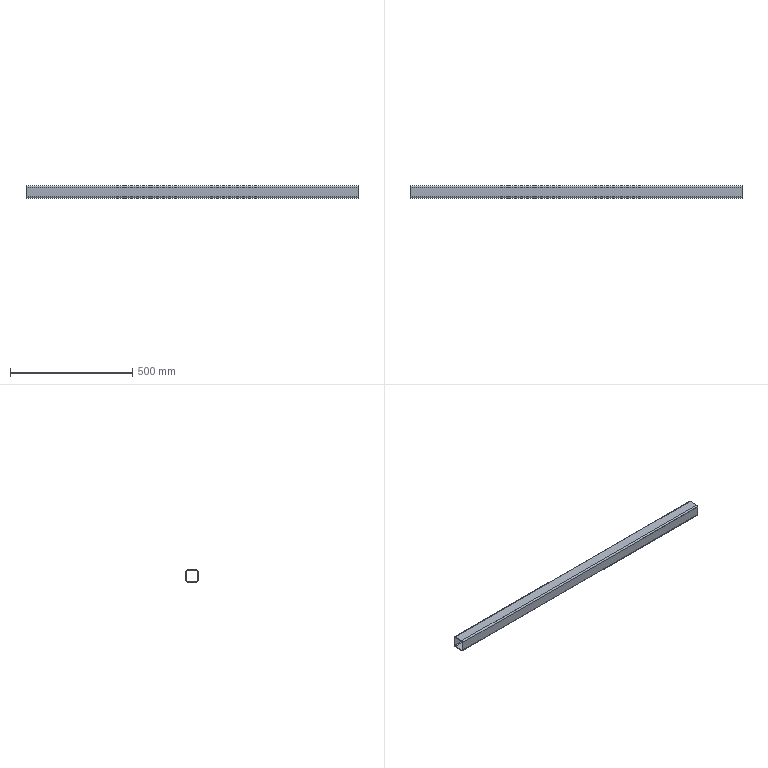Part | STEP file | VD-SYL0380DJ1006_1_1-5_VD-SYL03 | 1 solid | 18 faces | box 1360 x 50 x 50 mm | volume 735519 mm3 | plane 10 | cylinder 8 | commonest cylinder face diameters 6 x4 12 x4
STEP:
#1=CARTESIAN_POINT('',(-680.,-47.,-19.));
#2=VERTEX_POINT('',#1);
#3=CARTESIAN_POINT('',(680.,-47.,-19.));
#4=VERTEX_POINT('',#3);
#5=CARTESIAN_POINT('',(-680.,-47.,-19.));
#6=DIRECTION('',(1.,0.,0.));
#7=VECTOR('',#6,1000.);
#8=LINE('',#5,#7);
#9=EDGE_CURVE('',#2,#4,#8,.T.);
#10=ORIENTED_EDGE('',*,*,#9,.F.);
#11=CARTESIAN_POINT('',(-680.,-47.,19.));
#12=VERTEX_POINT('',#11);
#13=CARTESIAN_POINT('',(-680.,-47.,-19.));
#14=DIRECTION('',(0.,0.,1.));
#15=VECTOR('',#14,1000.);
#16=LINE('',#13,#15);
#17=EDGE_CURVE('',#2,#12,#16,.T.);
#18=ORIENTED_EDGE('',*,*,#17,.T.);
#19=CARTESIAN_POINT('',(680.,-47.,19.));
#20=VERTEX_POINT('',#19);
#21=CARTESIAN_POINT('',(680.,-47.,19.));
#22=DIRECTION('',(-1.,0.,0.));
#23=VECTOR('',#22,1000.);
#24=LINE('',#21,#23);
#25=EDGE_CURVE('',#20,#12,#24,.T.);
#26=ORIENTED_EDGE('',*,*,#25,.F.);
#27=CARTESIAN_POINT('',(680.,-47.,-19.));
#28=DIRECTION('',(0.,0.,1.));
#29=VECTOR('',#28,1000.);
#30=LINE('',#27,#29);
#31=EDGE_CURVE('',#4,#20,#30,.T.);
#32=ORIENTED_EDGE('',*,*,#31,.F.);
#33=EDGE_LOOP('',(#10,#18,#26,#32));
#34=FACE_OUTER_BOUND('',#33,.T.);
#35=CARTESIAN_POINT('',(-680.,-47.,25.));
#36=DIRECTION('',(0.,-1.,0.));
#37=DIRECTION('',(0.,0.,-1.));
#38=AXIS2_PLACEMENT_3D('',#35,#36,#37);
#39=PLANE('',#38);
#40=ADVANCED_FACE('',(#34),#39,.F.);
#41=CARTESIAN_POINT('',(680.,-44.,-22.));
#42=VERTEX_POINT('',#41);
#43=CARTESIAN_POINT('',(680.,-44.,-19.));
#44=DIRECTION('',(-1.,0.,0.));
#45=DIRECTION('',(0.,0.,-1.));
#46=AXIS2_PLACEMENT_3D('',#43,#44,#45);
#47=CIRCLE('',#46,3.);
#48=EDGE_CURVE('',#42,#4,#47,.T.);
#49=ORIENTED_EDGE('',*,*,#48,.F.);
#50=CARTESIAN_POINT('',(-680.,-44.,-22.));
#51=VERTEX_POINT('',#50);
#52=CARTESIAN_POINT('',(680.,-44.,-22.));
#53=DIRECTION('',(-1.,0.,0.));
#54=VECTOR('',#53,1000.);
#55=LINE('',#52,#54);
#56=EDGE_CURVE('',#42,#51,#55,.T.);
#57=ORIENTED_EDGE('',*,*,#56,.T.);
#58=CARTESIAN_POINT('',(-680.,-44.,-19.));
#59=DIRECTION('',(1.,0.,0.));
#60=DIRECTION('',(0.,-1.,0.));
#61=AXIS2_PLACEMENT_3D('',#58,#59,#60);
#62=CIRCLE('',#61,3.);
#63=EDGE_CURVE('',#2,#51,#62,.T.);
#64=ORIENTED_EDGE('',*,*,#63,.F.);
#65=ORIENTED_EDGE('',*,*,#9,.T.);
#66=EDGE_LOOP('',(#49,#57,#64,#65));
#67=FACE_OUTER_BOUND('',#66,.T.);
#68=CARTESIAN_POINT('',(-680.,-44.,-19.));
#69=DIRECTION('',(-1.,0.,0.));
#70=DIRECTION('',(0.,0.,1.));
#71=AXIS2_PLACEMENT_3D('',#68,#69,#70);
#72=CYLINDRICAL_SURFACE('',#71,3.);
#73=ADVANCED_FACE('',(#67),#72,.F.);
#74=CARTESIAN_POINT('',(-680.,-6.,-22.));
#75=VERTEX_POINT('',#74);
#76=CARTESIAN_POINT('',(680.,-6.,-22.));
#77=VERTEX_POINT('',#76);
#78=CARTESIAN_POINT('',(-680.,-6.,-22.));
#79=DIRECTION('',(1.,0.,0.));
#80=VECTOR('',#79,1000.);
#81=LINE('',#78,#80);
#82=EDGE_CURVE('',#75,#77,#81,.T.);
#83=ORIENTED_EDGE('',*,*,#82,.F.);
#84=CARTESIAN_POINT('',(-680.,-6.,-22.));
#85=DIRECTION('',(0.,-1.,0.));
#86=VECTOR('',#85,1000.);
#87=LINE('',#84,#86);
#88=EDGE_CURVE('',#75,#51,#87,.T.);
#89=ORIENTED_EDGE('',*,*,#88,.T.);
#90=ORIENTED_EDGE('',*,*,#56,.F.);
#91=CARTESIAN_POINT('',(680.,-6.,-22.));
#92=DIRECTION('',(0.,-1.,0.));
#93=VECTOR('',#92,1000.);
#94=LINE('',#91,#93);
#95=EDGE_CURVE('',#77,#42,#94,.T.);
#96=ORIENTED_EDGE('',*,*,#95,.F.);
#97=EDGE_LOOP('',(#83,#89,#90,#96));
#98=FACE_OUTER_BOUND('',#97,.T.);
#99=CARTESIAN_POINT('',(-680.,-50.,-22.));
#100=DIRECTION('',(0.,0.,-1.));
#101=DIRECTION('',(0.,-1.,0.));
#102=AXIS2_PLACEMENT_3D('',#99,#100,#101);
#103=PLANE('',#102);
#104=ADVANCED_FACE('',(#98),#103,.F.);
#105=CARTESIAN_POINT('',(680.,-3.,-19.));
#106=VERTEX_POINT('',#105);
#107=CARTESIAN_POINT('',(680.,-6.,-19.));
#108=DIRECTION('',(-1.,0.,0.));
#109=DIRECTION('',(0.,1.,0.));
#110=AXIS2_PLACEMENT_3D('',#107,#108,#109);
#111=CIRCLE('',#110,3.);
#112=EDGE_CURVE('',#106,#77,#111,.T.);
#113=ORIENTED_EDGE('',*,*,#112,.F.);
#114=CARTESIAN_POINT('',(-680.,-3.,-19.));
#115=VERTEX_POINT('',#114);
#116=CARTESIAN_POINT('',(680.,-3.,-19.));
#117=DIRECTION('',(-1.,0.,0.));
#118=VECTOR('',#117,1000.);
#119=LINE('',#116,#118);
#120=EDGE_CURVE('',#106,#115,#119,.T.);
#121=ORIENTED_EDGE('',*,*,#120,.T.);
#122=CARTESIAN_POINT('',(-680.,-6.,-19.));
#123=DIRECTION('',(1.,0.,0.));
#124=DIRECTION('',(0.,0.,-1.));
#125=AXIS2_PLACEMENT_3D('',#122,#123,#124);
#126=CIRCLE('',#125,3.);
#127=EDGE_CURVE('',#75,#115,#126,.T.);
#128=ORIENTED_EDGE('',*,*,#127,.F.);
#129=ORIENTED_EDGE('',*,*,#82,.T.);
#130=EDGE_LOOP('',(#113,#121,#128,#129));
#131=FACE_OUTER_BOUND('',#130,.T.);
#132=CARTESIAN_POINT('',(-680.,-6.,-19.));
#133=DIRECTION('',(-1.,0.,0.));
#134=DIRECTION('',(0.,0.,1.));
#135=AXIS2_PLACEMENT_3D('',#132,#133,#134);
#136=CYLINDRICAL_SURFACE('',#135,3.);
#137=ADVANCED_FACE('',(#131),#136,.F.);
#138=CARTESIAN_POINT('',(-680.,-3.,19.));
#139=VERTEX_POINT('',#138);
#140=CARTESIAN_POINT('',(680.,-3.,19.));
#141=VERTEX_POINT('',#140);
#142=CARTESIAN_POINT('',(-680.,-3.,19.));
#143=DIRECTION('',(1.,0.,0.));
#144=VECTOR('',#143,1000.);
#145=LINE('',#142,#144);
#146=EDGE_CURVE('',#139,#141,#145,.T.);
#147=ORIENTED_EDGE('',*,*,#146,.F.);
#148=CARTESIAN_POINT('',(-680.,-3.,19.));
#149=DIRECTION('',(0.,0.,-1.));
#150=VECTOR('',#149,1000.);
#151=LINE('',#148,#150);
#152=EDGE_CURVE('',#139,#115,#151,.T.);
#153=ORIENTED_EDGE('',*,*,#152,.T.);
#154=ORIENTED_EDGE('',*,*,#120,.F.);
#155=CARTESIAN_POINT('',(680.,-3.,19.));
#156=DIRECTION('',(0.,0.,-1.));
#157=VECTOR('',#156,1000.);
#158=LINE('',#155,#157);
#159=EDGE_CURVE('',#141,#106,#158,.T.);
#160=ORIENTED_EDGE('',*,*,#159,.F.);
#161=EDGE_LOOP('',(#147,#153,#154,#160));
#162=FACE_OUTER_BOUND('',#161,.T.);
#163=CARTESIAN_POINT('',(-680.,-3.,-25.));
#164=DIRECTION('',(0.,1.,0.));
#165=DIRECTION('',(1.,0.,0.));
#166=AXIS2_PLACEMENT_3D('',#163,#164,#165);
#167=PLANE('',#166);
#168=ADVANCED_FACE('',(#162),#167,.F.);
#169=CARTESIAN_POINT('',(680.,-6.,22.));
#170=VERTEX_POINT('',#169);
#171=CARTESIAN_POINT('',(680.,-6.,19.));
#172=DIRECTION('',(-1.,0.,0.));
#173=DIRECTION('',(0.,0.,1.));
#174=AXIS2_PLACEMENT_3D('',#171,#172,#173);
#175=CIRCLE('',#174,3.);
#176=EDGE_CURVE('',#170,#141,#175,.T.);
#177=ORIENTED_EDGE('',*,*,#176,.F.);
#178=CARTESIAN_POINT('',(-680.,-6.,22.));
#179=VERTEX_POINT('',#178);
#180=CARTESIAN_POINT('',(680.,-6.,22.));
#181=DIRECTION('',(-1.,0.,0.));
#182=VECTOR('',#181,1000.);
#183=LINE('',#180,#182);
#184=EDGE_CURVE('',#170,#179,#183,.T.);
#185=ORIENTED_EDGE('',*,*,#184,.T.);
#186=CARTESIAN_POINT('',(-680.,-6.,19.));
#187=DIRECTION('',(1.,0.,0.));
#188=DIRECTION('',(0.,1.,0.));
#189=AXIS2_PLACEMENT_3D('',#186,#187,#188);
#190=CIRCLE('',#189,3.);
#191=EDGE_CURVE('',#139,#179,#190,.T.);
#192=ORIENTED_EDGE('',*,*,#191,.F.);
#193=ORIENTED_EDGE('',*,*,#146,.T.);
#194=EDGE_LOOP('',(#177,#185,#192,#193));
#195=FACE_OUTER_BOUND('',#194,.T.);
#196=CARTESIAN_POINT('',(-680.,-6.,19.));
#197=DIRECTION('',(-1.,0.,0.));
#198=DIRECTION('',(0.,0.,1.));
#199=AXIS2_PLACEMENT_3D('',#196,#197,#198);
#200=CYLINDRICAL_SURFACE('',#199,3.);
#201=ADVANCED_FACE('',(#195),#200,.F.);
#202=CARTESIAN_POINT('',(-680.,0.,19.));
#203=VERTEX_POINT('',#202);
#204=CARTESIAN_POINT('',(-680.,0.,-19.));
#205=VERTEX_POINT('',#204);
#206=CARTESIAN_POINT('',(-680.,0.,19.));
#207=DIRECTION('',(0.,0.,-1.));
#208=VECTOR('',#207,1000.);
#209=LINE('',#206,#208);
#210=EDGE_CURVE('',#203,#205,#209,.T.);
#211=ORIENTED_EDGE('',*,*,#210,.F.);
#212=CARTESIAN_POINT('',(680.,0.,19.));
#213=VERTEX_POINT('',#212);
#214=CARTESIAN_POINT('',(680.,0.,19.));
#215=DIRECTION('',(-1.,0.,0.));
#216=VECTOR('',#215,1000.);
#217=LINE('',#214,#216);
#218=EDGE_CURVE('',#213,#203,#217,.T.);
#219=ORIENTED_EDGE('',*,*,#218,.F.);
#220=CARTESIAN_POINT('',(680.,0.,-19.));
#221=VERTEX_POINT('',#220);
#222=CARTESIAN_POINT('',(680.,0.,-19.));
#223=DIRECTION('',(0.,0.,1.));
#224=VECTOR('',#223,1000.);
#225=LINE('',#222,#224);
#226=EDGE_CURVE('',#221,#213,#225,.T.);
#227=ORIENTED_EDGE('',*,*,#226,.F.);
#228=CARTESIAN_POINT('',(-680.,0.,-19.));
#229=DIRECTION('',(1.,0.,0.));
#230=VECTOR('',#229,1000.);
#231=LINE('',#228,#230);
#232=EDGE_CURVE('',#205,#221,#231,.T.);
#233=ORIENTED_EDGE('',*,*,#232,.F.);
#234=EDGE_LOOP('',(#211,#219,#227,#233));
#235=FACE_OUTER_BOUND('',#234,.T.);
#236=CARTESIAN_POINT('',(-680.,0.,-25.));
#237=DIRECTION('',(0.,1.,0.));
#238=DIRECTION('',(1.,0.,0.));
#239=AXIS2_PLACEMENT_3D('',#236,#237,#238);
#240=PLANE('',#239);
#241=ADVANCED_FACE('',(#235),#240,.T.);
#242=CARTESIAN_POINT('',(-680.,-50.,19.));
#243=VERTEX_POINT('',#242);
#244=CARTESIAN_POINT('',(680.,-50.,19.));
#245=VERTEX_POINT('',#244);
#246=CARTESIAN_POINT('',(-680.,-50.,19.));
#247=DIRECTION('',(1.,0.,0.));
#248=VECTOR('',#247,1000.);
#249=LINE('',#246,#248);
#250=EDGE_CURVE('',#243,#245,#249,.T.);
#251=ORIENTED_EDGE('',*,*,#250,.T.);
#252=CARTESIAN_POINT('',(680.,-44.,25.));
#253=VERTEX_POINT('',#252);
#254=CARTESIAN_POINT('',(680.,-44.,19.));
#255=DIRECTION('',(1.,0.,0.));
#256=DIRECTION('',(0.,0.,1.));
#257=AXIS2_PLACEMENT_3D('',#254,#255,#256);
#258=CIRCLE('',#257,6.);
#259=EDGE_CURVE('',#253,#245,#258,.T.);
#260=ORIENTED_EDGE('',*,*,#259,.F.);
#261=CARTESIAN_POINT('',(-680.,-44.,25.));
#262=VERTEX_POINT('',#261);
#263=CARTESIAN_POINT('',(680.,-44.,25.));
#264=DIRECTION('',(-1.,0.,0.));
#265=VECTOR('',#264,1000.);
#266=LINE('',#263,#265);
#267=EDGE_CURVE('',#253,#262,#266,.T.);
#268=ORIENTED_EDGE('',*,*,#267,.T.);
#269=CARTESIAN_POINT('',(-680.,-44.,19.));
#270=DIRECTION('',(-1.,0.,0.));
#271=DIRECTION('',(0.,-1.,0.));
#272=AXIS2_PLACEMENT_3D('',#269,#270,#271);
#273=CIRCLE('',#272,6.);
#274=EDGE_CURVE('',#243,#262,#273,.T.);
#275=ORIENTED_EDGE('',*,*,#274,.F.);
#276=EDGE_LOOP('',(#251,#260,#268,#275));
#277=FACE_OUTER_BOUND('',#276,.T.);
#278=CARTESIAN_POINT('',(-680.,-44.,19.));
#279=DIRECTION('',(-1.,0.,0.));
#280=DIRECTION('',(0.,0.,1.));
#281=AXIS2_PLACEMENT_3D('',#278,#279,#280);
#282=CYLINDRICAL_SURFACE('',#281,6.);
#283=ADVANCED_FACE('',(#277),#282,.T.);
#284=CARTESIAN_POINT('',(-680.,-50.,-19.));
#285=VERTEX_POINT('',#284);
#286=CARTESIAN_POINT('',(-680.,-50.,-19.));
#287=DIRECTION('',(0.,0.,1.));
#288=VECTOR('',#287,1000.);
#289=LINE('',#286,#288);
#290=EDGE_CURVE('',#285,#243,#289,.T.);
#291=ORIENTED_EDGE('',*,*,#290,.F.);
#292=CARTESIAN_POINT('',(680.,-50.,-19.));
#293=VERTEX_POINT('',#292);
#294=CARTESIAN_POINT('',(680.,-50.,-19.));
#295=DIRECTION('',(-1.,0.,0.));
#296=VECTOR('',#295,1000.);
#297=LINE('',#294,#296);
#298=EDGE_CURVE('',#293,#285,#297,.T.);
#299=ORIENTED_EDGE('',*,*,#298,.F.);
#300=CARTESIAN_POINT('',(680.,-50.,19.));
#301=DIRECTION('',(0.,0.,-1.));
#302=VECTOR('',#301,1000.);
#303=LINE('',#300,#302);
#304=EDGE_CURVE('',#245,#293,#303,.T.);
#305=ORIENTED_EDGE('',*,*,#304,.F.);
#306=ORIENTED_EDGE('',*,*,#250,.F.);
#307=EDGE_LOOP('',(#291,#299,#305,#306));
#308=FACE_OUTER_BOUND('',#307,.T.);
#309=CARTESIAN_POINT('',(-680.,-50.,25.));
#310=DIRECTION('',(0.,-1.,0.));
#311=DIRECTION('',(0.,0.,-1.));
#312=AXIS2_PLACEMENT_3D('',#309,#310,#311);
#313=PLANE('',#312);
#314=ADVANCED_FACE('',(#308),#313,.T.);
#315=CARTESIAN_POINT('',(-680.,-44.,-25.));
#316=VERTEX_POINT('',#315);
#317=CARTESIAN_POINT('',(680.,-44.,-25.));
#318=VERTEX_POINT('',#317);
#319=CARTESIAN_POINT('',(-680.,-44.,-25.));
#320=DIRECTION('',(1.,0.,0.));
#321=VECTOR('',#320,1000.);
#322=LINE('',#319,#321);
#323=EDGE_CURVE('',#316,#318,#322,.T.);
#324=ORIENTED_EDGE('',*,*,#323,.T.);
#325=CARTESIAN_POINT('',(680.,-44.,-19.));
#326=DIRECTION('',(1.,0.,0.));
#327=DIRECTION('',(0.,-1.,0.));
#328=AXIS2_PLACEMENT_3D('',#325,#326,#327);
#329=CIRCLE('',#328,6.);
#330=EDGE_CURVE('',#293,#318,#329,.T.);
#331=ORIENTED_EDGE('',*,*,#330,.F.);
#332=ORIENTED_EDGE('',*,*,#298,.T.);
#333=CARTESIAN_POINT('',(-680.,-44.,-19.));
#334=DIRECTION('',(-1.,0.,0.));
#335=DIRECTION('',(0.,0.,-1.));
#336=AXIS2_PLACEMENT_3D('',#333,#334,#335);
#337=CIRCLE('',#336,6.);
#338=EDGE_CURVE('',#316,#285,#337,.T.);
#339=ORIENTED_EDGE('',*,*,#338,.F.);
#340=EDGE_LOOP('',(#324,#331,#332,#339));
#341=FACE_OUTER_BOUND('',#340,.T.);
#342=CARTESIAN_POINT('',(-680.,-44.,-19.));
#343=DIRECTION('',(-1.,0.,0.));
#344=DIRECTION('',(0.,0.,1.));
#345=AXIS2_PLACEMENT_3D('',#342,#343,#344);
#346=CYLINDRICAL_SURFACE('',#345,6.);
#347=ADVANCED_FACE('',(#341),#346,.T.);
#348=CARTESIAN_POINT('',(-680.,-6.,-25.));
#349=VERTEX_POINT('',#348);
#350=CARTESIAN_POINT('',(-680.,-6.,-25.));
#351=DIRECTION('',(0.,-1.,0.));
#352=VECTOR('',#351,1000.);
#353=LINE('',#350,#352);
#354=EDGE_CURVE('',#349,#316,#353,.T.);
#355=ORIENTED_EDGE('',*,*,#354,.F.);
#356=CARTESIAN_POINT('',(680.,-6.,-25.));
#357=VERTEX_POINT('',#356);
#358=CARTESIAN_POINT('',(680.,-6.,-25.));
#359=DIRECTION('',(-1.,0.,0.));
#360=VECTOR('',#359,1000.);
#361=LINE('',#358,#360);
#362=EDGE_CURVE('',#357,#349,#361,.T.);
#363=ORIENTED_EDGE('',*,*,#362,.F.);
#364=CARTESIAN_POINT('',(680.,-44.,-25.));
#365=DIRECTION('',(0.,1.,0.));
#366=VECTOR('',#365,1000.);
#367=LINE('',#364,#366);
#368=EDGE_CURVE('',#318,#357,#367,.T.);
#369=ORIENTED_EDGE('',*,*,#368,.F.);
#370=ORIENTED_EDGE('',*,*,#323,.F.);
#371=EDGE_LOOP('',(#355,#363,#369,#370));
#372=FACE_OUTER_BOUND('',#371,.T.);
#373=CARTESIAN_POINT('',(-680.,-50.,-25.));
#374=DIRECTION('',(0.,0.,-1.));
#375=DIRECTION('',(0.,-1.,0.));
#376=AXIS2_PLACEMENT_3D('',#373,#374,#375);
#377=PLANE('',#376);
#378=ADVANCED_FACE('',(#372),#377,.T.);
#379=ORIENTED_EDGE('',*,*,#232,.T.);
#380=CARTESIAN_POINT('',(680.,-6.,-19.));
#381=DIRECTION('',(1.,0.,0.));
#382=DIRECTION('',(0.,0.,-1.));
#383=AXIS2_PLACEMENT_3D('',#380,#381,#382);
#384=CIRCLE('',#383,6.);
#385=EDGE_CURVE('',#357,#221,#384,.T.);
#386=ORIENTED_EDGE('',*,*,#385,.F.);
#387=ORIENTED_EDGE('',*,*,#362,.T.);
#388=CARTESIAN_POINT('',(-680.,-6.,-19.));
#389=DIRECTION('',(-1.,0.,0.));
#390=DIRECTION('',(0.,1.,0.));
#391=AXIS2_PLACEMENT_3D('',#388,#389,#390);
#392=CIRCLE('',#391,6.);
#393=EDGE_CURVE('',#205,#349,#392,.T.);
#394=ORIENTED_EDGE('',*,*,#393,.F.);
#395=EDGE_LOOP('',(#379,#386,#387,#394));
#396=FACE_OUTER_BOUND('',#395,.T.);
#397=CARTESIAN_POINT('',(-680.,-6.,-19.));
#398=DIRECTION('',(-1.,0.,0.));
#399=DIRECTION('',(0.,0.,1.));
#400=AXIS2_PLACEMENT_3D('',#397,#398,#399);
#401=CYLINDRICAL_SURFACE('',#400,6.);
#402=ADVANCED_FACE('',(#396),#401,.T.);
#403=CARTESIAN_POINT('',(-680.,-44.,22.));
#404=VERTEX_POINT('',#403);
#405=CARTESIAN_POINT('',(-680.,-44.,19.));
#406=DIRECTION('',(1.,0.,0.));
#407=DIRECTION('',(0.,0.,1.));
#408=AXIS2_PLACEMENT_3D('',#405,#406,#407);
#409=CIRCLE('',#408,3.);
#410=EDGE_CURVE('',#404,#12,#409,.T.);
#411=ORIENTED_EDGE('',*,*,#410,.T.);
#412=ORIENTED_EDGE('',*,*,#17,.F.);
#413=ORIENTED_EDGE('',*,*,#63,.T.);
#414=ORIENTED_EDGE('',*,*,#88,.F.);
#415=ORIENTED_EDGE('',*,*,#127,.T.);
#416=ORIENTED_EDGE('',*,*,#152,.F.);
#417=ORIENTED_EDGE('',*,*,#191,.T.);
#418=CARTESIAN_POINT('',(-680.,-44.,22.));
#419=DIRECTION('',(0.,1.,0.));
#420=VECTOR('',#419,1000.);
#421=LINE('',#418,#420);
#422=EDGE_CURVE('',#404,#179,#421,.T.);
#423=ORIENTED_EDGE('',*,*,#422,.F.);
#424=EDGE_LOOP('',(#411,#412,#413,#414,#415,#416,#417,#423));
#425=FACE_BOUND('',#424,.T.);
#426=ORIENTED_EDGE('',*,*,#354,.T.);
#427=ORIENTED_EDGE('',*,*,#338,.T.);
#428=ORIENTED_EDGE('',*,*,#290,.T.);
#429=ORIENTED_EDGE('',*,*,#274,.T.);
#430=CARTESIAN_POINT('',(-680.,-6.,25.));
#431=VERTEX_POINT('',#430);
#432=CARTESIAN_POINT('',(-680.,-44.,25.));
#433=DIRECTION('',(0.,1.,0.));
#434=VECTOR('',#433,1000.);
#435=LINE('',#432,#434);
#436=EDGE_CURVE('',#262,#431,#435,.T.);
#437=ORIENTED_EDGE('',*,*,#436,.T.);
#438=CARTESIAN_POINT('',(-680.,-6.,19.));
#439=DIRECTION('',(-1.,0.,0.));
#440=DIRECTION('',(0.,0.,1.));
#441=AXIS2_PLACEMENT_3D('',#438,#439,#440);
#442=CIRCLE('',#441,6.);
#443=EDGE_CURVE('',#431,#203,#442,.T.);
#444=ORIENTED_EDGE('',*,*,#443,.T.);
#445=ORIENTED_EDGE('',*,*,#210,.T.);
#446=ORIENTED_EDGE('',*,*,#393,.T.);
#447=EDGE_LOOP('',(#426,#427,#428,#429,#437,#444,#445,#446));
#448=FACE_OUTER_BOUND('',#447,.T.);
#449=CARTESIAN_POINT('',(-680.,-25.,23.5));
#450=DIRECTION('',(-1.,0.,0.));
#451=DIRECTION('',(0.,0.,1.));
#452=AXIS2_PLACEMENT_3D('',#449,#450,#451);
#453=PLANE('',#452);
#454=ADVANCED_FACE('',(#425,#448),#453,.T.);
#455=CARTESIAN_POINT('',(680.,-6.,25.));
#456=VERTEX_POINT('',#455);
#457=CARTESIAN_POINT('',(-680.,-6.,25.));
#458=DIRECTION('',(1.,0.,0.));
#459=VECTOR('',#458,1000.);
#460=LINE('',#457,#459);
#461=EDGE_CURVE('',#431,#456,#460,.T.);
#462=ORIENTED_EDGE('',*,*,#461,.T.);
#463=CARTESIAN_POINT('',(680.,-6.,19.));
#464=DIRECTION('',(1.,0.,0.));
#465=DIRECTION('',(0.,1.,0.));
#466=AXIS2_PLACEMENT_3D('',#463,#464,#465);
#467=CIRCLE('',#466,6.);
#468=EDGE_CURVE('',#213,#456,#467,.T.);
#469=ORIENTED_EDGE('',*,*,#468,.F.);
#470=ORIENTED_EDGE('',*,*,#218,.T.);
#471=ORIENTED_EDGE('',*,*,#443,.F.);
#472=EDGE_LOOP('',(#462,#469,#470,#471));
#473=FACE_OUTER_BOUND('',#472,.T.);
#474=CARTESIAN_POINT('',(-680.,-6.,19.));
#475=DIRECTION('',(-1.,0.,0.));
#476=DIRECTION('',(0.,0.,1.));
#477=AXIS2_PLACEMENT_3D('',#474,#475,#476);
#478=CYLINDRICAL_SURFACE('',#477,6.);
#479=ADVANCED_FACE('',(#473),#478,.T.);
#480=ORIENTED_EDGE('',*,*,#436,.F.);
#481=ORIENTED_EDGE('',*,*,#267,.F.);
#482=CARTESIAN_POINT('',(680.,-6.,25.));
#483=DIRECTION('',(0.,-1.,0.));
#484=VECTOR('',#483,1000.);
#485=LINE('',#482,#484);
#486=EDGE_CURVE('',#456,#253,#485,.T.);
#487=ORIENTED_EDGE('',*,*,#486,.F.);
#488=ORIENTED_EDGE('',*,*,#461,.F.);
#489=EDGE_LOOP('',(#480,#481,#487,#488));
#490=FACE_OUTER_BOUND('',#489,.T.);
#491=CARTESIAN_POINT('',(-680.,0.,25.));
#492=DIRECTION('',(0.,0.,1.));
#493=DIRECTION('',(1.,0.,0.));
#494=AXIS2_PLACEMENT_3D('',#491,#492,#493);
#495=PLANE('',#494);
#496=ADVANCED_FACE('',(#490),#495,.T.);
#497=ORIENTED_EDGE('',*,*,#48,.T.);
#498=ORIENTED_EDGE('',*,*,#31,.T.);
#499=CARTESIAN_POINT('',(680.,-44.,22.));
#500=VERTEX_POINT('',#499);
#501=CARTESIAN_POINT('',(680.,-44.,19.));
#502=DIRECTION('',(-1.,0.,0.));
#503=DIRECTION('',(0.,-1.,0.));
#504=AXIS2_PLACEMENT_3D('',#501,#502,#503);
#505=CIRCLE('',#504,3.);
#506=EDGE_CURVE('',#20,#500,#505,.T.);
#507=ORIENTED_EDGE('',*,*,#506,.T.);
#508=CARTESIAN_POINT('',(680.,-44.,22.));
#509=DIRECTION('',(0.,1.,0.));
#510=VECTOR('',#509,1000.);
#511=LINE('',#508,#510);
#512=EDGE_CURVE('',#500,#170,#511,.T.);
#513=ORIENTED_EDGE('',*,*,#512,.T.);
#514=ORIENTED_EDGE('',*,*,#176,.T.);
#515=ORIENTED_EDGE('',*,*,#159,.T.);
#516=ORIENTED_EDGE('',*,*,#112,.T.);
#517=ORIENTED_EDGE('',*,*,#95,.T.);
#518=EDGE_LOOP('',(#497,#498,#507,#513,#514,#515,#516,#517));
#519=FACE_BOUND('',#518,.T.);
#520=ORIENTED_EDGE('',*,*,#259,.T.);
#521=ORIENTED_EDGE('',*,*,#304,.T.);
#522=ORIENTED_EDGE('',*,*,#330,.T.);
#523=ORIENTED_EDGE('',*,*,#368,.T.);
#524=ORIENTED_EDGE('',*,*,#385,.T.);
#525=ORIENTED_EDGE('',*,*,#226,.T.);
#526=ORIENTED_EDGE('',*,*,#468,.T.);
#527=ORIENTED_EDGE('',*,*,#486,.T.);
#528=EDGE_LOOP('',(#520,#521,#522,#523,#524,#525,#526,#527));
#529=FACE_OUTER_BOUND('',#528,.T.);
#530=CARTESIAN_POINT('',(680.,-25.,23.5));
#531=DIRECTION('',(-1.,0.,0.));
#532=DIRECTION('',(0.,0.,1.));
#533=AXIS2_PLACEMENT_3D('',#530,#531,#532);
#534=PLANE('',#533);
#535=ADVANCED_FACE('',(#519,#529),#534,.F.);
#536=CARTESIAN_POINT('',(-680.,-44.,22.));
#537=DIRECTION('',(1.,0.,0.));
#538=VECTOR('',#537,1000.);
#539=LINE('',#536,#538);
#540=EDGE_CURVE('',#404,#500,#539,.T.);
#541=ORIENTED_EDGE('',*,*,#540,.F.);
#542=ORIENTED_EDGE('',*,*,#422,.T.);
#543=ORIENTED_EDGE('',*,*,#184,.F.);
#544=ORIENTED_EDGE('',*,*,#512,.F.);
#545=EDGE_LOOP('',(#541,#542,#543,#544));
#546=FACE_OUTER_BOUND('',#545,.T.);
#547=CARTESIAN_POINT('',(-680.,0.,22.));
#548=DIRECTION('',(0.,0.,1.));
#549=DIRECTION('',(1.,0.,0.));
#550=AXIS2_PLACEMENT_3D('',#547,#548,#549);
#551=PLANE('',#550);
#552=ADVANCED_FACE('',(#546),#551,.F.);
#553=ORIENTED_EDGE('',*,*,#506,.F.);
#554=ORIENTED_EDGE('',*,*,#25,.T.);
#555=ORIENTED_EDGE('',*,*,#410,.F.);
#556=ORIENTED_EDGE('',*,*,#540,.T.);
#557=EDGE_LOOP('',(#553,#554,#555,#556));
#558=FACE_OUTER_BOUND('',#557,.T.);
#559=CARTESIAN_POINT('',(-680.,-44.,19.));
#560=DIRECTION('',(-1.,0.,0.));
#561=DIRECTION('',(0.,0.,1.));
#562=AXIS2_PLACEMENT_3D('',#559,#560,#561);
#563=CYLINDRICAL_SURFACE('',#562,3.);
#564=ADVANCED_FACE('',(#558),#563,.F.);
#565=CLOSED_SHELL('',(#40,#73,#104,#137,#168,#201,#241,#283,#314,#347,#378,#402,#454,#479,#496,#535,#552,#564));
#566=MANIFOLD_SOLID_BREP('',#565);
#567=CARTESIAN_POINT('',(0.,0.,0.));
#568=DIRECTION('',(0.,0.,1.));
#569=DIRECTION('',(1.,0.,0.));
#570=AXIS2_PLACEMENT_3D('',#567,#568,#569);
#571=(LENGTH_UNIT()NAMED_UNIT(*)SI_UNIT(.MILLI.,.METRE.));
#572=UNCERTAINTY_MEASURE_WITH_UNIT(LENGTH_MEASURE(0.00001),#571,'','');
#573=(NAMED_UNIT(*)PLANE_ANGLE_UNIT()SI_UNIT($,.RADIAN.));
#574=(NAMED_UNIT(*)SI_UNIT($,.STERADIAN.)SOLID_ANGLE_UNIT());
#575=(GEOMETRIC_REPRESENTATION_CONTEXT(3)GLOBAL_UNCERTAINTY_ASSIGNED_CONTEXT((#572))GLOBAL_UNIT_ASSIGNED_CONTEXT((#571,#573,#574))REPRESENTATION_CONTEXT('',''));
#576=ADVANCED_BREP_SHAPE_REPRESENTATION('',(#566,#570),#575);